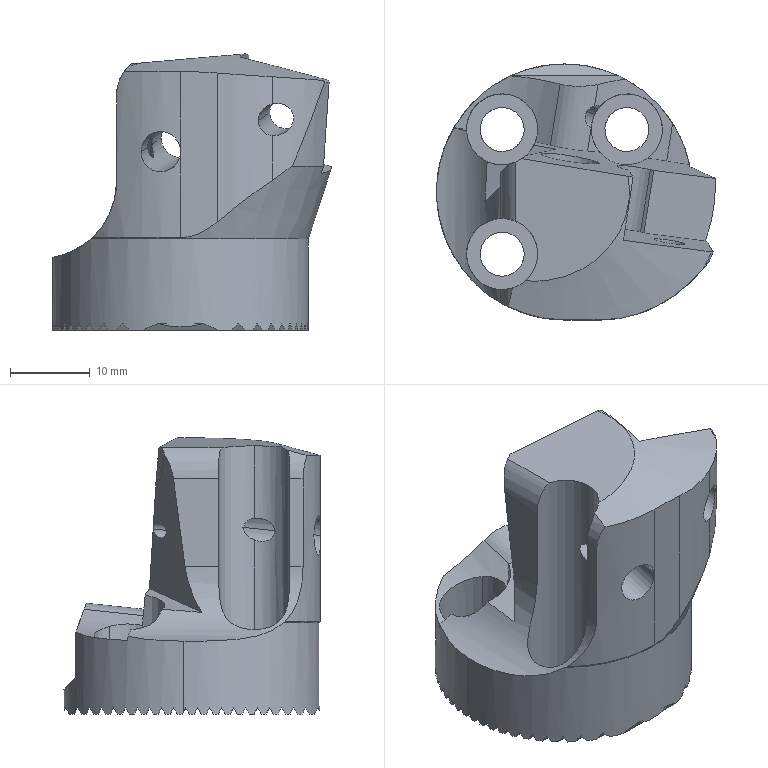NC program | Mastercam | posted with a generic post
Lines 3434 to 4113 of 7888:
(6 FEMR |TOOL - 5|DIA. OFF. - 5|LEN. - 5|TOOL DIA. - 6.)
N6924 T5 M6
N6926 G0 G54 G90 X22.689 Y25.292 C9. B-84. S3500 M3
N6928 G43 H5 Z48.807
N6930 Z.807
N6932 G1 Z-.943 F2000.
N6934 X22.31 Y24.394 Z-1.095 F1500.
N6936 G3 X22.204 Y23.869 Z-1.178 I1.243 J-.525
N6938 X22.207 Y23.77 Z-1.193 I1.349
N6940 G1 X22.229 Y23.466
N6942 G3 X22.664 Y23.422 I.435 J2.11
N6944 X22.751 Y23.423 J2.154
N6946 X25.986 Y23.592 I-.978 J49.933
N6948 X27.403 Y23.694 I-63.102 J886.628
N6950 G1 X27.606 Y23.708
N6952 X31.837 Y24.015
N6954 G2 X31.925 Y24.016 I.088 J-3.459
N6956 X34.127 Y23.225 J-3.46
N6958 X35.476 Y21.508 I-3.172 J-3.88
N6960 X36.337 Y19.149 I-12.706 J-5.974
N6962 X38.194 Y12.097 I-548.301 J-148.184
N6964 G1 X38.391 Y12.148
N6966 X38.588 Y12.2
N6968 G3 X39.145 Y12.497 Z-1.109 I-.339 J1.306
N6970 G1 X39.874 Y13.145 Z-.98
N6972 G3 X40.067 Y13.337 Z-.943 I-1.597 J1.796
N6974 X40.681 Y14.941 I-1.79 J1.604
N6976 X40.282 Y16.267 I-2.404
N6978 G1 X35.594 Y23.357 F9500.
N6980 G3 X33.132 Y24.873 I-2.864 J-1.895
N6982 G1 X23.875 Y25.964
N6984 G3 X23.741 Y25.972 I-.134 J-1.133
N6986 X22.825 Y25.511 J-1.141
N6988 X22.69 Y25.275 Z-.98 I.916 J-.68 F1500.
N6990 G1 X22.311 Y24.377 Z-1.109
N6992 G3 X22.204 Y23.851 Z-1.18 I1.244 J-.526
N6994 X22.208 Y23.753 Z-1.193 I1.351
N6996 G1 X22.23 Y23.449
N6998 X22.38 Y23.395
N7000 G3 X23.501 Y23.32 I1.121 J8.392
N7002 X24.044 Y23.338 J8.467
N7004 X30.035 Y23.735 I-13.266 J245.641
N7006 G1 X30.238 Y23.75
N7008 G2 X31.198 Y23.802 I.96 J-8.845
N7010 X31.506 Y23.797 J-8.897
N7012 X34.466 Y22.32 I-.355 J-4.417
N7014 X35.771 Y20.156 I-5.189 J-4.606
N7016 X36.663 Y17.344 I-24.364 J-9.273
N7018 X37.934 Y12.53 I-528.675 J-142.124
N7020 G3 X38.101 Y12.073 I7.045 J2.32
N7022 G1 X38.298 Y12.124
N7024 X38.495 Y12.175
N7026 G3 X39.053 Y12.473 Z-1.109 I-.339 J1.307
N7028 G1 X39.781 Y13.121 Z-.98
N7030 G3 X39.974 Y13.313 Z-.943 I-1.594 J1.794
N7032 X40.587 Y14.915 I-1.787 J1.602 F9500.
N7034 X40.126 Y16.329 I-2.4
N7036 G1 X35.137 Y23.168
N7038 G3 X33.083 Y24.501 I-2.77 J-2.02
N7040 G1 X24.704 Y26.29
N7042 G3 X24.332 Y26.329 I-.372 J-1.741
N7044 X22.817 Y25.483 J-1.78
N7046 X22.693 Y25.241 Z-.98 I1.515 J-.934 F1500.
N7048 G1 X22.313 Y24.343 Z-1.109
N7050 G3 X22.207 Y23.818 Z-1.18 I1.244 J-.525
N7052 X22.211 Y23.72 Z-1.193 I1.35
N7054 G1 X22.233 Y23.415
N7056 X22.234 Y23.399
N7058 G3 X23.119 Y23.24 I.989 J2.959
N7060 X24.032 Y23.222 I.913 J22.728
N7062 X25.831 Y23.293 J22.746
N7064 X30.347 Y23.603 I-26.998 J427.037
N7066 G2 X30.634 Y23.611 I.287 J-4.952
N7068 X34.533 Y21.717 J-4.96
N7070 X35.77 Y19.539 I-6.172 J-4.943
N7072 X36.769 Y16.343 I-28.424 J-10.648
N7074 X37.643 Y13.046 I-386.556 J-104.218
N7076 G3 X38.016 Y12.051 I5.206 J1.383
N7078 G1 X38.213 Y12.102
N7080 X38.41 Y12.153
N7082 G3 X38.967 Y12.451 Z-1.109 I-.339 J1.307
N7084 G1 X39.696 Y13.099 Z-.98
N7086 G3 X39.889 Y13.29 Z-.943 I-1.641 J1.846
N7088 X40.525 Y14.945 I-1.834 J1.655 F9500.
N7090 X39.947 Y16.535 I-2.47
N7092 G1 X34.35 Y23.197
N7094 G3 X32.303 Y24.395 I-2.703 J-2.271
N7096 G1 X24.086 Y25.948
N7098 G3 X23.853 Y25.97 I-.233 J-1.235
N7100 X22.828 Y25.439 J-1.257
N7102 X22.695 Y25.202 Z-.98 I1.025 J-.726 F1500.
N7104 G1 X22.316 Y24.304 Z-1.109
N7106 G3 X22.21 Y23.779 Z-1.18 I1.244 J-.525
N7108 X22.213 Y23.68 Z-1.193 I1.35
N7110 G1 X22.236 Y23.376
N7112 X22.237 Y23.357
N7114 G3 X23.081 Y23.157 I1.066 J2.613
N7116 X24.427 Y23.101 I1.346 J16.269
N7118 X25.505 Y23.137 J16.325
N7120 X29.787 Y23.41 I-8.866 J173.072
N7122 G2 X30.153 Y23.422 I.366 J-5.516
N7124 X32.806 Y22.743 J-5.528
N7126 X35.005 Y20.533 I-3.048 J-5.231
N7128 X36.123 Y17.954 I-10.779 J-6.203
N7130 X37.308 Y13.719 I-86.534 J-26.499
N7132 G3 X37.788 Y12.304 I8.176 J1.984
N7134 G2 X37.934 Y12.03 I-10.185 J-5.609
N7136 G1 X38.131 Y12.081
N7138 X38.328 Y12.132
N7140 G3 X38.885 Y12.43 Z-1.109 I-.339 J1.307
N7142 G1 X39.614 Y13.077 Z-.98
N7144 G3 X39.807 Y13.269 Z-.943 I-1.619 J1.822
N7146 X40.432 Y14.899 I-1.812 J1.63 F9500.
N7148 X39.835 Y16.497 I-2.437
N7150 G1 X34.218 Y22.96
N7152 G3 X32.506 Y24.035 I-2.627 J-2.283
N7154 G1 X24.739 Y26.151
N7156 G3 X24.286 Y26.212 I-.453 J-1.663
N7158 X22.824 Y25.4 J-1.724
N7160 X22.699 Y25.158 Z-.98 I1.462 J-.912 F1500.
N7162 G1 X22.319 Y24.26 Z-1.109
N7164 G3 X22.213 Y23.735 Z-1.18 I1.244 J-.525
N7166 X22.217 Y23.637 Z-1.193 I1.35
N7168 G1 X22.239 Y23.332
N7170 X22.24 Y23.312
N7172 G3 X23.05 Y23.078 I1.131 J2.387
N7174 X24.664 Y22.979 I1.614 J13.094
N7176 X25.396 Y22.999 J13.193
N7178 X29.23 Y23.22 I-4.831 J117.045
N7180 G2 X29.675 Y23.235 I.445 J-6.436
N7182 X31.856 Y22.856 J-6.451
N7184 X34.593 Y20.669 I-2.233 J-5.602
N7186 X35.889 Y18.053 I-8.883 J-6.03
N7188 X36.983 Y14.348 I-49.334 J-16.582
N7190 G3 X37.551 Y12.573 I13.656 J3.39
N7192 X37.854 Y12.009 I3.182 J1.347
N7194 G1 X38.051 Y12.06
N7196 X38.248 Y12.111
N7198 G3 X38.806 Y12.409 Z-1.109 I-.339 J1.307
N7200 G1 X39.534 Y13.057 Z-.98
N7202 G3 X39.728 Y13.248 Z-.943 I-1.692 J1.904
N7204 X40.39 Y14.961 I-1.886 J1.713 F9500.
N7206 X39.634 Y16.771 I-2.548
N7208 G1 X33.296 Y23.045
N7210 G3 X31.681 Y23.973 I-2.56 J-2.586
N7212 G1 X24.387 Y25.935
N7214 G3 X24.016 Y25.984 I-.371 J-1.378
N7216 X22.831 Y25.352 J-1.427
N7218 X22.702 Y25.112 Z-.98 I1.185 J-.795 F1500.
N7220 G1 X22.323 Y24.214 Z-1.109
N7222 G3 X22.217 Y23.689 Z-1.18 I1.243 J-.525
N7224 X22.22 Y23.591 Z-1.193 I1.349
N7226 G1 X22.242 Y23.286
N7228 X22.244 Y23.265
N7230 G3 X23.024 Y23.001 I1.181 J2.205
N7232 X24.756 Y22.857 I1.732 J10.372
N7234 X25.116 Y22.863 J10.516
N7236 X28.686 Y23.035 I-1.603 J70.711
N7238 G2 X29.227 Y23.054 I.541 J-7.556
N7240 X31.103 Y22.818 J-7.575
N7242 X34.344 Y20.554 I-1.676 J-5.85
N7244 X35.721 Y17.945 I-8.407 J-6.107
N7246 X36.752 Y14.616 I-37.471 J-13.421
N7248 G3 X37.388 Y12.669 I14.489 J3.662
N7250 X37.776 Y11.989 I3.119 J1.325
N7252 G1 X37.973 Y12.04
N7254 X38.169 Y12.091
N7256 G3 X38.727 Y12.388 Z-1.109 I-.339 J1.307
N7258 G1 X39.456 Y13.036 Z-.98
N7260 G3 X39.649 Y13.227 Z-.943 I-1.727 J1.943
N7262 X40.328 Y14.979 I-1.92 J1.752 F9500.
N7264 X39.471 Y16.909 I-2.599
N7266 G1 X32.737 Y22.991
N7268 G3 X31.273 Y23.804 I-2.489 J-2.756
N7270 G1 X24.274 Y25.814
N7272 G3 X23.912 Y25.865 I-.362 J-1.259
N7274 X22.837 Y25.302 J-1.31
N7276 X22.705 Y25.064 Z-.98 I1.075 J-.747 F1500.
N7278 G1 X22.326 Y24.166 Z-1.109
N7280 G3 X22.22 Y23.641 Z-1.18 I1.244 J-.525
N7282 X22.224 Y23.543 Z-1.193 I1.35
N7284 G1 X22.246 Y23.238
N7286 X22.247 Y23.216
N7288 G3 X23.13 Y22.897 I1.303 J2.225
N7290 X25.034 Y22.733 I1.904 J10.982
N7292 X25.401 Y22.739 J11.146
N7294 X28.391 Y22.863 I-1.215 J65.38
N7296 G2 X28.868 Y22.877 I.477 J-7.911
N7298 X30.893 Y22.615 J-7.925
N7300 X34.194 Y20.316 I-1.78 J-6.077
N7302 X35.594 Y17.729 I-8.292 J-6.159
N7304 X36.594 Y14.608 I-33.709 J-12.528
N7306 G3 X37.26 Y12.685 I13.361 J3.546
N7308 X37.698 Y11.968 I3.095 J1.399
N7310 G1 X37.895 Y12.019
N7312 X38.092 Y12.071
N7314 G3 X38.649 Y12.368 Z-1.109 I-.34 J1.306
N7316 G1 X39.378 Y13.016 Z-.98
N7318 G3 X39.571 Y13.207 Z-.943 I-1.747 J1.965
N7320 X40.26 Y14.981 I-1.94 J1.774 F9500.
N7322 X39.332 Y16.985 I-2.629
N7324 G1 X32.357 Y22.904
N7326 G3 X31.121 Y23.602 I-2.43 J-2.863
N7328 G1 X24.499 Y25.822
N7330 G3 X24.04 Y25.897 I-.459 J-1.37
N7332 X22.838 Y25.254 J-1.445
N7334 X22.709 Y25.014 Z-.98 I1.202 J-.802 F1500.
N7336 G1 X22.33 Y24.116 Z-1.109
N7338 G3 X22.224 Y23.591 Z-1.18 I1.244 J-.525
N7340 X22.227 Y23.493 Z-1.193 I1.35
N7342 G1 X22.249 Y23.188
N7344 X22.251 Y23.165
N7346 G3 X23.107 Y22.819 I1.346 J2.099
N7348 X25.143 Y22.611 I2.036 J9.849
N7350 X25.324 Y22.613 J10.057
N7352 X28.1 Y22.696 I-.309 J56.833
N7354 G2 X28.519 Y22.707 I.419 J-8.285
N7356 X30.686 Y22.418 J-8.296
N7358 X33.962 Y20.194 I-1.844 J-6.241
N7360 X35.425 Y17.619 I-7.972 J-6.235
N7362 X36.408 Y14.695 I-30.788 J-11.978
N7364 G3 X37.1 Y12.765 I13.851 J3.873
N7366 X37.62 Y11.948 I3.089 J1.394
N7368 G1 X37.817 Y11.999
N7370 X38.014 Y12.05
N7372 G3 X38.571 Y12.348 Z-1.109 I-.339 J1.307
N7374 G1 X39.3 Y12.996 Z-.98
N7376 G3 X39.493 Y13.187 Z-.943 I-1.656 J1.863
N7378 X40.137 Y14.859 I-1.849 J1.672 F9500.
N7380 X39.305 Y16.718 I-2.493
N7382 G1 X32.833 Y22.5
N7384 G3 X31.779 Y23.152 I-2.373 J-2.655
N7386 G1 X24.922 Y25.887
N7388 G3 X24.289 Y26.008 I-.633 J-1.589
N7390 X22.838 Y25.205 J-1.71
N7392 X22.713 Y24.963 Z-.98 I1.451 J-.907 F1500.
N7394 G1 X22.334 Y24.065 Z-1.109
N7396 G3 X22.228 Y23.54 Z-1.18 I1.243 J-.525
N7398 X22.231 Y23.442 Z-1.193 I1.349
N7400 G1 X22.253 Y23.137
N7402 X22.255 Y23.113
N7404 G3 X23.086 Y22.743 I1.383 J1.987
N7406 X25.236 Y22.49 I2.15 J8.999
N7408 X25.254 Y22.489 J9.252
N7410 X25.755 Y22.486 I.501 J46.821
N7412 X27.815 Y22.532 J46.824
N7414 G2 X28.126 Y22.537 I.311 J-9.212
N7416 X30.322 Y22.272 J-9.217
N7418 X33.921 Y19.838 I-1.771 J-6.497
N7420 X35.437 Y17.066 I-8.791 J-6.608
N7422 X36.395 Y14.238 I-43.073 J-16.176
N7424 G3 X37.12 Y12.499 I9.002 J2.73
N7426 X37.542 Y11.928 I2.505 J1.412
N7428 G1 X37.739 Y11.979
N7430 X37.936 Y12.03
N7432 G3 X38.494 Y12.328 Z-1.109 I-.339 J1.307
N7434 G1 X39.222 Y12.976 Z-.98
N7436 G3 X39.416 Y13.167 Z-.943 I-1.696 J1.909
N7438 X40.08 Y14.885 I-1.89 J1.718 F9500.
N7440 X39.145 Y16.861 I-2.554
N7442 G1 X32.288 Y22.479
N7444 G3 X31.379 Y23.024 I-2.313 J-2.823
N7446 G1 X24.806 Y25.765
N7448 G3 X24.19 Y25.888 I-.616 J-1.476
N7450 X22.843 Y25.151 J-1.599
N7452 X22.717 Y24.911 Z-.98 I1.347 J-.862 F1500.
N7454 G1 X22.337 Y24.013 Z-1.109
N7456 G3 X22.231 Y23.488 Z-1.18 I1.244 J-.525
N7458 X22.235 Y23.389 Z-1.193 I1.35
N7460 G1 X22.257 Y23.085
N7462 X22.259 Y23.059
N7464 G3 X23.066 Y22.667 I1.438 J1.934
N7466 X25.189 Y22.369 I2.238 J8.241
N7468 X26.281 Y22.355 I1.092 J43.35
N7470 X27.535 Y22.374 J43.364
N7472 G2 X27.753 Y22.376 I.218 J-9.825
N7474 X30.123 Y22.086 J-9.827
N7476 X33.79 Y19.605 I-1.847 J-6.68
N7478 X35.315 Y16.856 I-8.886 J-6.725
N7480 X36.236 Y14.252 I-50.738 J-19.416
N7482 G3 X36.994 Y12.513 I9.018 J2.895
N7484 X37.465 Y11.908 I2.518 J1.475
N7486 G1 X37.662 Y11.959
N7488 X37.859 Y12.01
N7490 G3 X38.416 Y12.308 Z-1.109 I-.34 J1.307
N7492 G1 X39.145 Y12.955 Z-.98
N7494 G3 X39.338 Y13.147 Z-.943 I-1.695 J1.907
N7496 X40.001 Y14.862 I-1.888 J1.715 F9500.
N7498 X39.027 Y16.867 I-2.551
N7500 G1 X32.083 Y22.325
N7502 G3 X31.322 Y22.785 I-2.252 J-2.864
N7504 G1 X24.842 Y25.692
N7506 G3 X24.19 Y25.831 I-.652 J-1.455
N7508 X22.847 Y25.098 J-1.594
N7510 X22.721 Y24.857 Z-.98 I1.343 J-.861 F1500.
N7512 G1 X22.341 Y23.959 Z-1.109
N7514 G3 X22.235 Y23.434 Z-1.18 I1.244 J-.525
N7516 X22.239 Y23.336 Z-1.193 I1.35
N7518 G1 X22.261 Y23.031
N7520 X22.263 Y23.005
N7522 G3 X23.167 Y22.553 I1.601 J2.074
N7524 X25.304 Y22.244 I2.312 J8.434
N7526 X27.053 Y22.216 I1.749 J54.493
N7528 X27.49 Y22.218 J54.521
N7530 G2 X30.224 Y21.816 I-.005 J-9.546
N7532 X33.832 Y19.152 I-2.275 J-6.854
N7534 X35.279 Y16.437 I-9.86 J-7.001
N7536 X36.202 Y13.928 I-69.696 J-27.054
N7538 G3 X36.992 Y12.337 I6.926 J2.449
N7540 X37.387 Y11.888 I2.118 J1.462
N7542 G1 X37.584 Y11.939
N7544 X37.781 Y11.99
N7546 G3 X38.338 Y12.288 Z-1.109 I-.339 J1.307
N7548 G1 X39.067 Y12.935 Z-.98
N7550 G3 X39.261 Y13.127 Z-.943 I-1.694 J1.907
N7552 X39.924 Y14.842 I-1.888 J1.715 F9500.
N7554 X38.907 Y16.879 I-2.551
N7556 G1 X31.867 Y22.18
N7558 G3 X31.255 Y22.552 I-2.192 J-2.911
N7560 G1 X24.884 Y25.619
N7562 G3 X24.193 Y25.777 I-.691 J-1.436
N7564 X22.851 Y25.043 J-1.594
N7566 X22.725 Y24.803 Z-.98 I1.342 J-.86 F1500.
N7568 G1 X22.345 Y23.905 Z-1.109
N7570 G3 X22.238 Y23.379 Z-1.18 I1.244 J-.526
N7572 X22.243 Y23.281 Z-1.193 I1.351
N7574 G1 X22.265 Y22.977
N7576 X22.267 Y22.949
N7578 G3 X23.146 Y22.477 I1.574 J1.873
N7580 X25.247 Y22.126 I2.393 J7.872
N7582 X27.448 Y22.06 I2.54 J47.785
N7584 G2 X30.32 Y21.537 I-.188 J-9.185
N7586 X33.705 Y18.927 I-2.657 J-6.945
N7588 X35.16 Y16.239 I-10.091 J-7.198
N7590 X36.043 Y13.947 I-64.228 J-26.078
N7592 G3 X36.864 Y12.352 I7.102 J2.646
N7594 X37.18 Y11.986 I1.86 J1.284
N7596 X37.352 Y11.879 I.399 J.448
N7598 G1 X37.549 Y11.93
N7600 G3 X38.107 Y12.227 Z-1.109 I-.339 J1.306
N7602 G1 X38.835 Y12.875 Z-.98
N7604 G3 X39.028 Y13.067 Z-.943 I-1.566 J1.762
N7606 X39.627 Y14.637 I-1.759 J1.57 F9500.
N7608 X38.675 Y16.53 I-2.358
N7610 G1 X26.307 Y25.722
N7612 G3 X24.901 Y26.187 I-1.406 J-1.892
N7614 X22.849 Y24.991 J-2.357
N7616 X22.729 Y24.747 Z-.98 I2.052 J-1.161 F1500.
N7618 G1 X22.349 Y23.849 Z-1.109
N7620 G3 X22.243 Y23.324 Z-1.18 I1.244 J-.525
N7622 X22.247 Y23.226 Z-1.193 I1.35
N7624 G1 X22.269 Y22.921
N7626 X22.271 Y22.893
N7628 G3 X23.126 Y22.4 I1.597 J1.786
N7630 X25.195 Y22.01 I2.471 J7.421
N7632 X27.41 Y21.901 I3.803 J54.561
N7634 G2 X30.256 Y21.314 I-.463 J-9.439
N7636 X33.577 Y18.71 I-2.858 J-7.064
N7638 X35.039 Y16.052 I-10.388 J-7.446
N7640 X35.88 Y13.973 I-90.198 J-37.681
N7642 G3 X36.732 Y12.37 I7.327 J2.866
N7644 X37.245 Y11.851 I1.951 J1.414
N7646 G1 X37.441 Y11.902
N7648 X37.638 Y11.953
N7650 G3 X38.196 Y12.251 Z-1.109 I-.339 J1.307
N7652 G1 X38.925 Y12.898 Z-.98
N7654 G3 X39.117 Y13.09 Z-.943 I-1.568 J1.764
N7656 X39.717 Y14.662 I-1.76 J1.572 F9500.
N7658 X38.75 Y16.567 I-2.36
N7660 G1 X26.301 Y25.677
N7662 G3 X24.907 Y26.133 I-1.394 J-1.904
N7664 X22.853 Y24.935 J-2.36
N7666 X22.733 Y24.691 Z-.98 I2.054 J-1.162 F1500.
N7668 G1 X22.354 Y23.793 Z-1.109
N7670 G3 X22.247 Y23.267 Z-1.18 I1.243 J-.526
N7672 X22.251 Y23.169 Z-1.193 I1.35
N7674 G1 X22.273 Y22.865
N7676 X22.275 Y22.835
N7678 G3 X23.107 Y22.325 I1.597 J1.67
N7680 X25.147 Y21.896 I2.551 J7.057
N7682 X27.138 Y21.761 I4.287 J48.562
N7684 G2 X29.77 Y21.255 I-.633 J-10.386
N7686 X33.528 Y18.39 I-2.623 J-7.339
N7688 X34.963 Y15.773 I-11.379 J-7.939
N7690 G3 X35.967 Y13.452 I60.803 J24.923
N7692 X36.766 Y12.188 I4.917 J2.227
N7694 X37.161 Y11.829 I1.846 J1.63
N7696 G1 X37.358 Y11.88
N7698 X37.554 Y11.931
N7700 G3 X38.112 Y12.229 Z-1.109 I-.339 J1.307
N7702 G1 X38.841 Y12.876 Z-.98
N7704 G3 X39.033 Y13.069 Z-.943 I-1.561 J1.756
N7706 X39.629 Y14.632 I-1.753 J1.563 F9500.
N7708 X38.67 Y16.526 I-2.349
N7710 G1 X26.292 Y25.613
N7712 G3 X24.901 Y26.069 I-1.391 J-1.894
N7714 X22.857 Y24.877 J-2.35
N7716 X22.737 Y24.633 Z-.98 I2.044 J-1.158 F1500.
N7718 G1 X22.358 Y23.735 Z-1.109
N7720 G3 X22.252 Y23.21 Z-1.18 I1.243 J-.525
N7722 X22.255 Y23.112 Z-1.193 I1.349
N7724 G1 X22.277 Y22.807
N7726 X22.279 Y22.777
N7728 G3 X23.088 Y22.25 I1.62 J1.602
N7730 X25.102 Y21.782 I2.634 J6.764
N7732 X27.101 Y21.606 I5.812 J54.447
N7734 G2 X29.99 Y20.932 I-.852 J-10.188
N7736 X33.393 Y18.194 I-3.162 J-7.413
N7738 X34.839 Y15.613 I-11.678 J-8.24
N7740 X35.42 Y14.299 I-105.398 J-47.372
N7742 G3 X36.328 Y12.588 I9.612 J4.002
N7744 X37.078 Y11.807 I2.381 J1.539
N7746 G1 X37.275 Y11.859
N7748 X37.472 Y11.91
N7750 G3 X38.03 Y12.207 Z-1.109 I-.339 J1.306
N7752 G1 X38.758 Y12.855 Z-.98
N7754 G3 X38.951 Y13.047 Z-.943 I-1.553 J1.748
N7756 X39.544 Y14.603 I-1.746 J1.556 F9500.
N7758 X38.591 Y16.486 I-2.339
N7760 G1 X26.282 Y25.549
N7762 G3 X24.896 Y26.004 I-1.386 J-1.884
N7764 X22.861 Y24.819 J-2.339
N7766 X22.741 Y24.575 Z-.98 I2.035 J-1.154 F1500.
N7768 G1 X22.362 Y23.677 Z-1.109
N7770 G3 X22.256 Y23.152 Z-1.18 I1.244 J-.525
N7772 X22.259 Y23.053 Z-1.193 I1.35
N7774 G1 X22.281 Y22.749
N7776 X22.284 Y22.718
N7778 G3 X23.07 Y22.176 I1.634 J1.529
N7780 X24.89 Y21.693 I2.591 J6.093
N7782 X27.065 Y21.45 I5.884 J42.831
N7784 G2 X29.926 Y20.717 I-1.106 J-10.272
N7786 X33.274 Y17.982 I-3.371 J-7.542
N7788 X34.726 Y15.44 I-12.24 J-8.681
N7790 X35.243 Y14.325 I-139.105 J-65.111
N7792 G3 X36.186 Y12.605 I9.968 J4.35
N7794 X36.996 Y11.786 I2.54 J1.703
N7796 G1 X37.193 Y11.837
N7798 X37.39 Y11.888
N7800 G3 X37.948 Y12.186 Z-1.109 I-.339 J1.307
N7802 G1 X38.676 Y12.834 Z-.98
N7804 G3 X38.869 Y13.026 Z-.943 I-1.546 J1.74
N7806 X39.458 Y14.574 I-1.739 J1.548 F9500.
N7808 X38.513 Y16.446 I-2.328
N7810 G1 X26.273 Y25.483
N7812 G3 X24.89 Y25.938 I-1.383 J-1.873
N7814 X22.866 Y24.76 J-2.328
N7816 X22.746 Y24.516 Z-.98 I2.024 J-1.15 F1500.
N7818 G1 X22.366 Y23.618 Z-1.109
N7820 G3 X22.26 Y23.093 Z-1.18 I1.244 J-.525
N7822 X22.264 Y22.994 Z-1.193 I1.35
N7824 G1 X22.286 Y22.69
N7826 X22.288 Y22.657
N7828 G3 X23.052 Y22.102 I1.629 J1.436
N7830 X24.851 Y21.584 I2.672 J5.896
N7832 X26.799 Y21.326 I7.481 J49.167
N7834 G2 X29.592 Y20.622 I-1.339 J-11.199
N7836 X33.155 Y17.774 I-3.3 J-7.781
N7838 X34.708 Y15.081 I-13.376 J-9.51
N7840 G3 X35.797 Y12.985 I21.154 J9.656
N7842 X36.728 Y11.888 I3.411 J1.952
N7844 X36.783 Y11.85 I.61 J.825
N7846 X36.952 Y11.775 I.326 J.504
N7848 G1 X37.149 Y11.826
N7850 G3 X37.706 Y12.123 Z-1.109 I-.34 J1.306
N7852 G1 X38.435 Y12.771 Z-.98
N7854 G3 X38.627 Y12.963 Z-.943 I-1.531 J1.723
N7856 X39.209 Y14.494 I-1.723 J1.531 F9500.
N7858 X38.291 Y16.335 I-2.305
N7860 G1 X26.26 Y25.4
N7862 G3 X24.873 Y25.864 I-1.387 J-1.841
N7864 X22.87 Y24.7 J-2.305
N7866 X22.75 Y24.456 Z-.98 I2.003 J-1.141 F1500.
N7868 G1 X22.371 Y23.558 Z-1.109
N7870 G3 X22.265 Y23.033 Z-1.18 I1.243 J-.525
N7872 X22.268 Y22.934 Z-1.193 I1.349
N7874 G1 X22.29 Y22.63
N7876 X22.332 Y22.543
N7878 G3 X23.373 Y21.872 I1.998 J1.957
N7880 X25.339 Y21.386 I3.033 J8.051
N7882 X26.541 Y21.21 I18.661 J123.126
N7884 G2 X29.265 Y20.526 I-1.655 J-12.355
N7886 X33.035 Y17.573 I-3.237 J-8.017
N7888 X34.599 Y14.925 I-14.202 J-10.175
N7890 G1 X34.692 Y14.741
N7892 G3 X35.804 Y12.762 I15.149 J7.209
N7894 X36.576 Y11.914 I2.928 J1.888
N7896 X36.844 Y11.747 I1.673 J2.382
N7898 G1 X37.041 Y11.798
N7900 X37.238 Y11.849
N7902 G3 X37.795 Y12.146 Z-1.109 I-.34 J1.307
N7904 G1 X38.524 Y12.794 Z-.98
N7906 G3 X38.708 Y12.994 Z-.943 I-.897 J1.009
N7908 X38.977 Y13.803 I-1.081 J.809 F9500.
N7910 X38.429 Y14.889 I-1.35
N7912 G1 X24.8 Y24.956
N7914 G3 X23.998 Y25.22 I-.802 J-1.086
N7916 X22.885 Y24.634 J-1.35
N7918 X22.754 Y24.395 Z-.98 I1.113 J-.764 F1500.
N7920 G1 X22.375 Y23.497 Z-1.109
N7922 G3 X22.269 Y22.972 Z-1.18 I1.244 J-.525
N7924 X22.272 Y22.874 Z-1.193 I1.35
N7926 G1 X22.295 Y22.569
N7928 X22.335 Y22.481
N7930 G3 X23.351 Y21.792 I2.01 J1.869
N7932 X25.303 Y21.266 I3.18 J7.931
N7934 G2 X27.669 Y20.824 I-5.836 J-37.797
N7936 X33.069 Y17.168 I-1.95 J-8.696
N7938 X34.586 Y14.596 I-17.82 J-12.246
N7940 G3 X35.731 Y12.669 I13.476 J6.703
N7942 X36.599 Y11.812 I2.799 J1.966
N7944 X36.803 Y11.736 I.309 J.515
N7946 G1 X37. Y11.787
N7948 G3 X37.557 Y12.085 Z-1.109 I-.34 J1.307
N7950 G1 X38.286 Y12.732 Z-.98
N7952 G3 X38.47 Y12.932 Z-.943 I-.897 J1.009
N7954 X38.739 Y13.741 I-1.081 J.809 F9500.
N7956 X38.201 Y14.82 I-1.35
N7958 G1 X24.814 Y24.887
N7960 G3 X24.003 Y25.158 I-.811 J-1.079
N7962 X22.889 Y24.572 J-1.35
N7964 X22.759 Y24.333 Z-.98 I1.114 J-.764 F1500.
N7966 G1 X22.38 Y23.435 Z-1.109
N7968 G3 X22.274 Y22.91 Z-1.18 I1.243 J-.525
N7970 X22.277 Y22.812 Z-1.193 I1.349
N7972 G1 X22.299 Y22.507
N7974 X22.338 Y22.418
N7976 G3 X23.329 Y21.712 I2.004 J1.763
N7978 X25.269 Y21.147 I3.334 J7.834
N7980 X26.253 Y20.959 I24.433 J125.769
N7982 G2 X28.882 Y20.237 I-2.432 J-13.998
N7984 X32.796 Y17.188 I-3.454 J-8.47
N7986 X34.384 Y14.634 I-16.27 J-11.884
N7988 G3 X35.569 Y12.695 I14.7 J7.661
N7990 X36.438 Y11.836 I3.042 J2.204
N7992 X36.683 Y11.705 I2.013 J3.482
N7994 G1 X36.88 Y11.756
N7996 X37.077 Y11.807
N7998 G3 X37.635 Y12.105 Z-1.109 I-.339 J1.307
N8000 G1 X38.363 Y12.752 Z-.98
N8002 G3 X38.547 Y12.952 Z-.943 I-.897 J1.009
N8004 X38.816 Y13.761 I-1.081 J.809 F9500.
N8006 X38.271 Y14.846 I-1.35
N8008 G1 X24.811 Y24.83
N8010 G3 X24.007 Y25.096 I-.804 J-1.084
N8012 X22.894 Y24.509 J-1.35
N8014 X22.763 Y24.271 Z-.98 I1.113 J-.763 F1500.
N8016 G1 X22.384 Y23.373 Z-1.109
N8018 G3 X22.278 Y22.848 Z-1.18 I1.244 J-.525
N8020 X22.281 Y22.749 Z-1.193 I1.35
N8022 G1 X22.304 Y22.445
N8024 X22.341 Y22.354
N8026 G3 X23.307 Y21.631 I2.01 J1.681
N8028 X25.235 Y21.027 I3.49 J7.748
N8030 X26.217 Y20.818 I17.445 J79.618
N8032 G2 X29.071 Y19.935 I-2.569 J-13.365
N8034 X32.675 Y17.005 I-3.996 J-8.598
N8036 X34.277 Y14.497 I-17.866 J-13.173
N8038 G3 X35.491 Y12.611 I13.387 J7.286
N8040 X36.403 Y11.775 I2.798 J2.133
N8042 X36.658 Y11.698 I.295 J.522
N8044 G1 X36.855 Y11.749
N8046 G3 X37.412 Y12.047 Z-1.109 I-.34 J1.307
N8048 G1 X38.141 Y12.695 Z-.98
N8050 G3 X38.325 Y12.895 Z-.943 I-.897 J1.009
N8052 X38.594 Y13.704 I-1.081 J.809 F9500.
N8054 X38.057 Y14.782 I-1.35
N8056 G1 X24.825 Y24.76
N8058 G3 X24.012 Y25.032 I-.813 J-1.078
N8060 X22.898 Y24.446 J-1.35
N8062 X22.768 Y24.208 Z-.98 I1.114 J-.764 F1500.
N8064 G1 X22.389 Y23.309 Z-1.109
N8066 G3 X22.283 Y22.784 Z-1.18 I1.244 J-.525
N8068 X22.286 Y22.686 Z-1.193 I1.35
N8070 G1 X22.308 Y22.382
N8072 X22.344 Y22.289
N8074 G3 X23.287 Y21.551 I2.015 J1.603
N8076 X25.201 Y20.906 I3.649 J7.673
N8078 X26.18 Y20.676 I20.034 J82.969
N8080 G2 X29.002 Y19.744 I-2.935 J-13.616
N8082 X32.555 Y16.828 I-4.272 J-8.828
N8084 X34.171 Y14.365 I-19.351 J-14.459
N8086 G3 X35.414 Y12.529 I12.263 J6.963
N8088 X36.322 Y11.75 I2.485 J1.977
N8090 X36.581 Y11.691 I.259 J.541
N8092 X36.64 Y11.694 J.6
N8094 G1 X36.57 Y12.287 Z-1.114
N8096 G3 X36.263 Y13.534 Z-.943 I-5.143 J-.606
N8098 X35.367 Y15.042 I-4.836 J-1.853 F9500.
N8100 G1 X27.042 Y24.803
N8102 G3 X25.111 Y25.694 I-1.931 J-1.647
N8104 X22.892 Y24.388 J-2.538
N8106 X22.773 Y24.143 Z-.98 I2.219 J-1.232 F1500.
N8108 G1 X22.394 Y23.245 Z-1.109
N8110 G3 X22.288 Y22.72 Z-1.18 I1.243 J-.525
N8112 X22.291 Y22.622 Z-1.193 I1.349
N8114 G1 X22.313 Y22.317
N8116 X22.348 Y22.223
N8118 G3 X23.267 Y21.471 I2.016 J1.525
N8120 X24.99 Y20.834 I3.665 J7.27
N8122 X26.353 Y20.479 I22.807 J84.858
N8124 G2 X29.173 Y19.431 I-3.149 J-12.788
N8126 X32.434 Y16.656 I-4.86 J-9.015
N8128 X34.065 Y14.239 I-21.067 J-15.971
N8130 G3 X35.335 Y12.452 I11.312 J6.695
N8132 X36.206 Y11.74 I2.335 J1.969
N8134 X36.272 Y11.713 I.497 J1.119
N8136 X36.486 Y11.674 I.214 J.561
N8138 X36.637 Y11.693 J.6
N8140 X37.195 Y11.99 Z-1.109 I-.339 J1.307
N8142 G1 X37.923 Y12.638 Z-.98
N8144 G3 X38.107 Y12.838 Z-.943 I-.897 J1.009
N8146 X38.376 Y13.647 I-1.081 J.809 F9500.
N8148 X37.844 Y14.721 I-1.35
N8150 G1 X24.839 Y24.627
N8152 G3 X24.021 Y24.903 I-.818 J-1.074
N8154 X22.908 Y24.317 J-1.35
N8156 X22.777 Y24.078 Z-.98 I1.113 J-.764 F1500.
N8158 G1 X22.398 Y23.18 Z-1.109
N8160 G3 X22.292 Y22.655 Z-1.18 I1.244 J-.525
N8162 X22.296 Y22.557 Z-1.193 I1.35
N8164 G1 X22.318 Y22.252
N8166 X22.351 Y22.157
N8168 G3 X23.248 Y21.39 I2.017 J1.45
N8170 X24.958 Y20.717 I3.819 J7.207
N8172 X26.313 Y20.334 I24.86 J85.283
N8174 G2 X29.332 Y19.111 I-3.422 J-12.781
N8176 X32.466 Y16.295 I-5.601 J-9.387
N8178 X34.066 Y13.955 I-28.782 J-21.389
N8180 G3 X35.349 Y12.281 I9.059 J5.617
N8182 X36.199 Y11.684 I1.747 J1.585
N8184 X36.398 Y11.65 I.199 J.567
N8186 X36.549 Y11.67 J.601
N8188 X37.106 Y11.967 Z-1.109 I-.34 J1.307
N8190 G1 X37.835 Y12.615 Z-.98
N8192 G3 X38.019 Y12.815 Z-.943 I-.897 J1.009
N8194 X38.288 Y13.624 I-1.081 J.809 F9500.
N8196 X37.757 Y14.697 I-1.35
N8198 G1 X24.845 Y24.56
N8200 G3 X24.026 Y24.837 I-.819 J-1.073
N8202 X22.913 Y24.251 J-1.35
N8204 X22.782 Y24.012 Z-.98 I1.113 J-.764 F1500.
N8206 G1 X22.403 Y23.114 Z-1.109
N8208 G3 X22.297 Y22.589 Z-1.18 I1.244 J-.525
N8210 X22.3 Y22.491 Z-1.193 I1.35
N8212 G1 X22.323 Y22.186
N8214 X22.355 Y22.089
N8216 G3 X23.229 Y21.308 I2.016 J1.378
N8218 X24.926 Y20.601 I3.974 J7.141
N8220 X26.272 Y20.189 I26.522 J84.357
N8222 G2 X29.249 Y18.925 I-3.823 J-13.137
N8224 X32.345 Y16.137 I-5.934 J-9.704
N8226 X33.962 Y13.841 I-32.612 J-24.683
N8228 G3 X35.268 Y12.215 I8.472 J5.469
N8230 X36.116 Y11.656 I1.719 J1.687
N8232 X36.308 Y11.624 I.192 J.569
N8234 X36.407 Y11.633 J.601
N8236 G1 X36.604 Y11.684
N8238 G3 X37.614 Y12.991 Z-.957 I-.34 J1.307
N8240 X37.61 Y13.098 Z-.943 I-1.35
N8242 X37.078 Y14.068 I-1.346 J-.107 F9500.
N8244 G1 X24.466 Y23.599
N8246 G3 X23.652 Y23.872 I-.814 J-1.077
N8248 X23.321 Y23.831 J-1.35
N8250 X22.302 Y22.522 Z-1.18 I.331 J-1.309 F1500.
N8252 X22.305 Y22.423 Z-1.193 I1.35
N8254 G1 X22.327 Y22.119
N8256 X22.358 Y22.02
N8258 G3 X23.212 Y21.226 I2.045 J1.341
N8260 X24.894 Y20.483 I4.13 J7.083
N8262 X26.23 Y20.045 I27.759 J82.256
N8264 G2 X29.164 Y18.742 I-4.186 J-13.389
N8266 X32.225 Y15.982 I-6.291 J-10.054
N8268 X33.859 Y13.73 I-37.564 J-28.966
N8270 G3 X35.091 Y12.239 I8.334 J5.635
N8272 X36.026 Y11.628 I1.822 J1.765
N8274 X36.205 Y11.601 I.179 J.573
N8276 X36.356 Y11.62 J.6
N8278 X37.366 Y12.926 Z-.957 I-.339 J1.306
N8280 X37.362 Y13.034 Z-.943 I-1.349